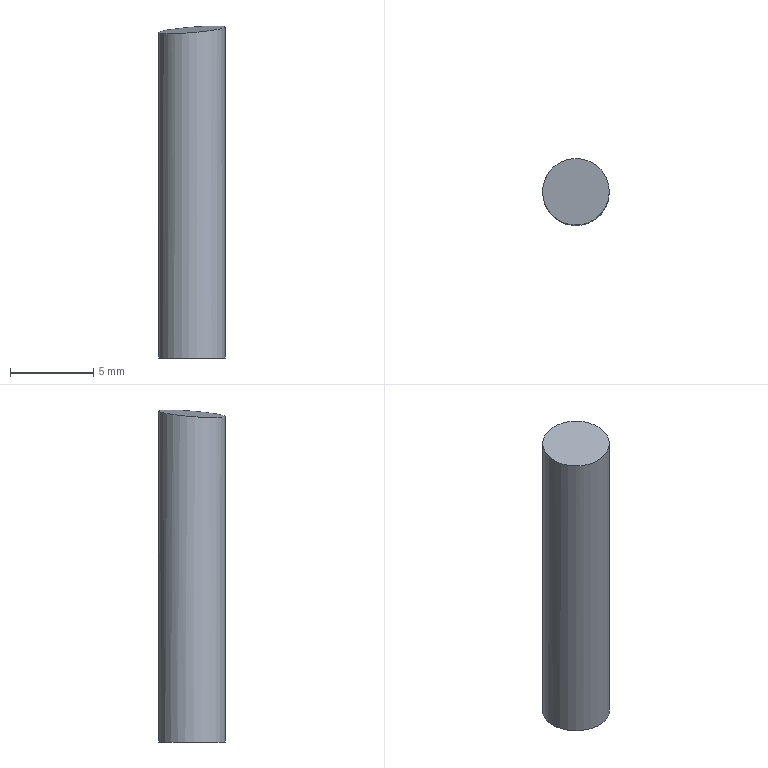Part | NX | features solid 2 | 1 solid | 3 faces | box 4 x 4 x 19.915 mm | volume 247.335 mm3 | plane 2 | cylinder 1 | commonest cylinder face diameters 4 x1
STEP:
#1=CARTESIAN_POINT('',(720.314,18.97,-15.));
#2=VERTEX_POINT('',#1);
#3=CARTESIAN_POINT('',(718.314,18.97,-15.));
#4=DIRECTION('',(0.,0.,1.));
#5=DIRECTION('',(1.,0.,0.));
#6=AXIS2_PLACEMENT_3D('',#3,#4,#5);
#7=CIRCLE('',#6,2.);
#8=EDGE_CURVE('',#2,#2,#7,.T.);
#9=ORIENTED_EDGE('',*,*,#8,.F.);
#10=EDGE_LOOP('',(#9));
#11=FACE_BOUND('',#10,.T.);
#12=CARTESIAN_POINT('',(718.314,18.97,-15.));
#13=DIRECTION('',(0.,0.,-1.));
#14=DIRECTION('',(-1.,0.,0.));
#15=AXIS2_PLACEMENT_3D('',#12,#13,#14);
#16=PLANE('',#15);
#17=ADVANCED_FACE('',(#11),#16,.T.);
#18=CARTESIAN_POINT('',(716.894,17.562,4.45));
#19=VERTEX_POINT('',#18);
#20=CARTESIAN_POINT('',(718.314,18.97,4.682));
#21=DIRECTION('',(0.08207,0.08131,-0.9933));
#22=DIRECTION('',(-0.7057,-0.6991,-0.1155));
#23=AXIS2_PLACEMENT_3D('',#20,#21,#22);
#24=ELLIPSE('',#23,2.013,2.);
#25=EDGE_CURVE('',#19,#19,#24,.T.);
#26=ORIENTED_EDGE('',*,*,#25,.F.);
#27=EDGE_LOOP('',(#26));
#28=FACE_BOUND('',#27,.T.);
#29=CARTESIAN_POINT('',(769.706,-95.382,-0.4319));
#30=DIRECTION('',(0.08207,0.08131,-0.9933));
#31=DIRECTION('',(0.9966,-0.01117,0.08143));
#32=AXIS2_PLACEMENT_3D('',#29,#30,#31);
#33=PLANE('',#32);
#34=ADVANCED_FACE('',(#28),#33,.F.);
#35=ORIENTED_EDGE('',*,*,#8,.T.);
#36=EDGE_LOOP('',(#35));
#37=FACE_BOUND('',#36,.T.);
#38=ORIENTED_EDGE('',*,*,#25,.T.);
#39=EDGE_LOOP('',(#38));
#40=FACE_BOUND('',#39,.T.);
#41=CARTESIAN_POINT('',(718.314,18.97,5.));
#42=DIRECTION('',(0.,0.,-1.));
#43=DIRECTION('',(-1.,0.,0.));
#44=AXIS2_PLACEMENT_3D('',#41,#42,#43);
#45=CYLINDRICAL_SURFACE('',#44,2.);
#46=ADVANCED_FACE('',(#37,#40),#45,.T.);
#47=CLOSED_SHELL('',(#17,#34,#46));
#48=MANIFOLD_SOLID_BREP('',#47);
#49=(LENGTH_UNIT()NAMED_UNIT(*)SI_UNIT(.MILLI.,.METRE.));
#50=UNCERTAINTY_MEASURE_WITH_UNIT(LENGTH_MEASURE(0.00001),#49,'','');
#51=(NAMED_UNIT(*)PLANE_ANGLE_UNIT()SI_UNIT($,.RADIAN.));
#52=(NAMED_UNIT(*)SI_UNIT($,.STERADIAN.)SOLID_ANGLE_UNIT());
#53=(GEOMETRIC_REPRESENTATION_CONTEXT(3)GLOBAL_UNCERTAINTY_ASSIGNED_CONTEXT((#50))GLOBAL_UNIT_ASSIGNED_CONTEXT((#49,#51,#52))REPRESENTATION_CONTEXT('',''));
#54=ADVANCED_BREP_SHAPE_REPRESENTATION('',(#48),#53);